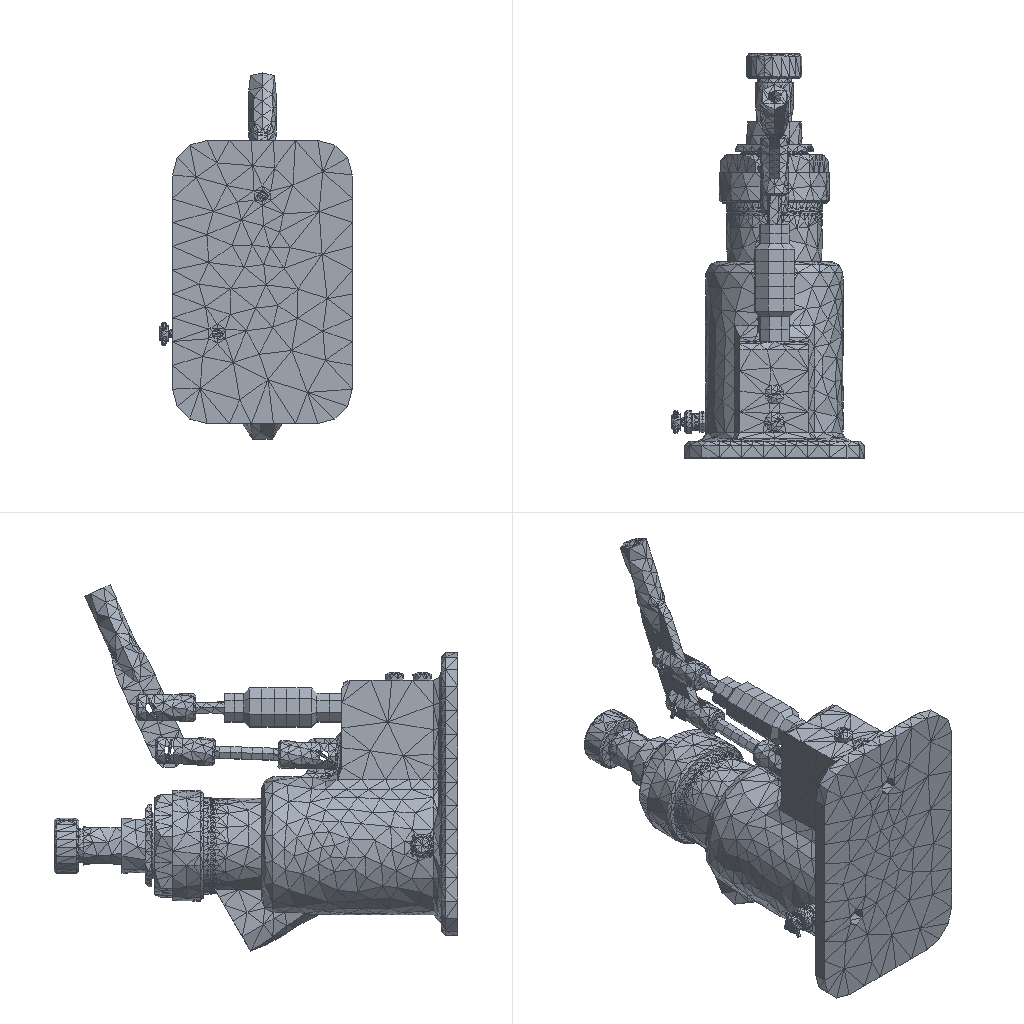Simulation study | ansys workbench
Ansys APDL input file, long lists of numbers shortened:
/batch
/config,noeldb,1     ! force off writing results to database
*get,_wallstrt,active,,time,wall
! ANSYS input file written by Workbench version 2022 R1
! File used for geometry attach:
/title,___--__ (B5)
! ****** Begin Custom Load Command Snippet ******
/COM, ACT Extensions:
/COM,     LSDYNA, 2021.1
/COM,
! ****** End   Custom Load Command Snippet ******
*DIM,_wb_ProjectScratch_dir,string,248
_wb_ProjectScratch_dir(1) = ''
*DIM,_wb_SolverFiles_dir,string,248
_wb_SolverFiles_dir(1) = ''
*DIM,_wb_userfiles_dir,string,248
_wb_userfiles_dir(1) = ''
/com,--- Data in consistent NMM units. See Solving Units in the help system for more information.
/units,MPA
/nopr
/wb,file,start              !  signify a WB generated input file
/prep7
! Turn off shape checking because checks already performed inside WB mesher.
! See help system for more information.
SHPP,OFF,,NOWARN
/nolist
etcon,set             ! allow ANSYS to choose best KEYOP's for 180x elements, resets any applicable keyopt to MAPDL defaults
/com,*********** Nodes for the whole assembly ***********
nblock,3,,64544
(1i9,3e20.9e3)
        1     2.522581875E+01    -4.240918474E+01     1.018764446E+02
! (58676 more lines like these left out)
-1
/wb,elem,start            !  set before creation of elements
/com,*********** Elements for Body 1 "3 - Caixa|Chamfer3" ***********
et,1,187
eblock,19,solid,,12883
(19i9)
        1        1        1        1        0        0        0        0       10        0    15841    34635    35994    34636    35272    49223    49227    49216    49218
! (25765 more lines like these left out)
-1
/com,*********** Elements for Body 2 "4 - Camisa|3/16 (0.1875) Diameter Hole1" ***********
et,2,187
eblock,19,solid,,1067
(19i9)
        2        2        2        2        0        0        0        0       10        0    10106    21478    21481    21733    21857    21878    21894    21881    21882
! (2133 more lines like these left out)
-1
/com,*********** Elements for Body 3 "2 - Porca especial|Cut-Revolve2" ***********
et,3,187
eblock,19,solid,,1009
(19i9)
        3        3        3        3        0        0        0        0       10        0     6814    15045    15047    15293    15279    16019    16039    16027    16025
! (2017 more lines like these left out)
-1
/com,*********** Elements for Body 4 "11 - Porca especial|Chamfer2" ***********
et,4,187
eblock,19,solid,,3371
(19i9)
        4        4        4        4        0        0        0        0       10        0    11173    24012    24701    24402    24248    26827    28868    26825    26824
! (6741 more lines like these left out)
-1
/com,*********** Elements for Body 5 "38 - Eixo Central|Chamfer1" ***********
et,5,187
eblock,19,solid,,853
(19i9)
        5        5        5        5        0        0        0        0       10        0     5961    13343    13573    13546    13550    13911    14889    13907    13908
! (1705 more lines like these left out)
-1
! (22 more sections like these left out)
/wb,elem,end               !  done creating elements
/com,*********** Send User Defined Coordinate System(s) ***********
csys,0
toffst,273.15,  ! Temperature offset from absolute zero
/com,*********** Set Reference Temperature ***********
tref,22.
/wb,mat,start              !  starting to send materials
/com,*********** Send Materials ***********
Temperature = 'TEMP' ! Temperature
MP,DENS,1,7.85e-09,	! tonne mm^-3
MP,ALPX,1,1.2e-05,	! C^-1
MP,C,1,434000000,	! mm^2 s^-2 C^-1
MP,KXX,1,60.5,	! tonne mm s^-3 C^-1
MP,RSVX,1,0.00017,	! ohm mm
MP,EX,1,200000,	! tonne s^-2 mm^-1
MP,NUXY,1,0.3,
MP,MURX,1,10000,
Temperature = 'TEMP' ! Temperature
MP,DENS,2,7.85e-09,	! tonne mm^-3
MP,ALPX,2,1.2e-05,	! C^-1
MP,C,2,434000000,	! mm^2 s^-2 C^-1
MP,KXX,2,60.5,	! tonne mm s^-3 C^-1
MP,RSVX,2,0.00017,	! ohm mm
MP,EX,2,200000,	! tonne s^-2 mm^-1
MP,NUXY,2,0.3,
MP,MURX,2,10000,
Temperature = 'TEMP' ! Temperature
MP,DENS,3,7.85e-09,	! tonne mm^-3
MP,ALPX,3,1.2e-05,	! C^-1
MP,C,3,434000000,	! mm^2 s^-2 C^-1
MP,KXX,3,60.5,	! tonne mm s^-3 C^-1
MP,RSVX,3,0.00017,	! ohm mm
MP,EX,3,200000,	! tonne s^-2 mm^-1
MP,NUXY,3,0.3,
MP,MURX,3,10000,
Temperature = 'TEMP' ! Temperature
MP,DENS,4,7.85e-09,	! tonne mm^-3
MP,ALPX,4,1.2e-05,	! C^-1
MP,C,4,434000000,	! mm^2 s^-2 C^-1
MP,KXX,4,60.5,	! tonne mm s^-3 C^-1
MP,RSVX,4,0.00017,	! ohm mm
MP,EX,4,200000,	! tonne s^-2 mm^-1
MP,NUXY,4,0.3,
MP,MURX,4,10000,
Temperature = 'TEMP' ! Temperature
MP,DENS,5,7.85e-09,	! tonne mm^-3
MP,ALPX,5,1.2e-05,	! C^-1
MP,C,5,434000000,	! mm^2 s^-2 C^-1
MP,KXX,5,60.5,	! tonne mm s^-3 C^-1
MP,RSVX,5,0.00017,	! ohm mm
MP,EX,5,200000,	! tonne s^-2 mm^-1
MP,NUXY,5,0.3,
MP,MURX,5,10000,
Temperature = 'TEMP' ! Temperature
MP,DENS,6,7.85e-09,	! tonne mm^-3
MP,ALPX,6,1.2e-05,	! C^-1
MP,C,6,434000000,	! mm^2 s^-2 C^-1
MP,KXX,6,60.5,	! tonne mm s^-3 C^-1
MP,RSVX,6,0.00017,	! ohm mm
MP,EX,6,200000,	! tonne s^-2 mm^-1
MP,NUXY,6,0.3,
MP,MURX,6,10000,
Temperature = 'TEMP' ! Temperature
MP,DENS,7,7.85e-09,	! tonne mm^-3
MP,ALPX,7,1.2e-05,	! C^-1
MP,C,7,434000000,	! mm^2 s^-2 C^-1
MP,KXX,7,60.5,	! tonne mm s^-3 C^-1
MP,RSVX,7,0.00017,	! ohm mm
MP,EX,7,200000,	! tonne s^-2 mm^-1
MP,NUXY,7,0.3,
MP,MURX,7,10000,
Temperature = 'TEMP' ! Temperature
MP,DENS,8,7.85e-09,	! tonne mm^-3
MP,ALPX,8,1.2e-05,	! C^-1
MP,C,8,434000000,	! mm^2 s^-2 C^-1
MP,KXX,8,60.5,	! tonne mm s^-3 C^-1
MP,RSVX,8,0.00017,	! ohm mm
MP,EX,8,200000,	! tonne s^-2 mm^-1
MP,NUXY,8,0.3,
MP,MURX,8,10000,
Temperature = 'TEMP' ! Temperature
MP,DENS,9,7.85e-09,	! tonne mm^-3
MP,ALPX,9,1.2e-05,	! C^-1
MP,C,9,434000000,	! mm^2 s^-2 C^-1
MP,KXX,9,60.5,	! tonne mm s^-3 C^-1
MP,RSVX,9,0.00017,	! ohm mm
MP,EX,9,200000,	! tonne s^-2 mm^-1
! (164 more lines like these left out)
/wb,mat,end                !  done sending materials
!************************* Model Summary ********************
!3 - Caixa|Chamfer3,	结构钢,	matid,	1
!4 - Camisa|3/16 (0.1875) Diameter Hole1,	结构钢,	matid,	2
!2 - Porca especial|Cut-Revolve2,	结构钢,	matid,	3
!11 - Porca especial|Chamfer2,	结构钢,	matid,	4
!38 - Eixo Central|Chamfer1,	结构钢,	matid,	5
!10 - Espiga|Cut-Extrude1,	结构钢,	matid,	6
!8 - Agulha|Chamfer2,	结构钢,	matid,	7
!9 - Parafuso da agulha|M6 Tapped Hole1,	结构钢,	matid,	8
!7 - Porca Trava|M12 Tapped Hole1,	结构钢,	matid,	9
!23 - Esfera|Revolve1,	结构钢,	matid,	10
!23 - Esfera|Revolve1[2],	结构钢,	matid,	11
!24 - Mola|Cut-Extrude1,	结构钢,	matid,	12
!24 - Mola|Cut-Extrude1[2],	结构钢,	matid,	13
!37 - Encaixa de alavanca|Cut-Extrude3,	结构钢,	matid,	14
!33 - Eixo de encaixe|Boss-Extrude2,	结构钢,	matid,	15
!37 - Encaixa de alavanca|Cut-Extrude3[2],	结构钢,	matid,	16
!36 - Alavanca|_10.0 (10) Diameter Hole1,	结构钢,	matid,	17
!37 - Encaixa de alavanca|Cut-Extrude3[3],	结构钢,	matid,	18
!30 - Eixo Injector|M6 Tapped Hole1,	结构钢,	matid,	19
!socket head cap screw_din_DIN 912 M6 x 20 --- 20N|Hex,	结构钢,	matid,	20
!split pin_din_DIN 94-2x10-C-St|ConeCut,	结构钢,	matid,	21
!split pin_din_DIN 94-2x10-C-St|ConeCut[2],	结构钢,	matid,	22
!split pin_din_DIN 94-2x10-C-St|ConeCut[3],	结构钢,	matid,	23
!22 - Luva do pist_o|_10.0 (10) Diameter Hole1,	结构钢,	matid,	24
!26 - Parafuso cabe_a redonda|Cut-Extrude1,	结构钢,	matid,	25
!26 - Parafuso cabe_a redonda|Cut-Extrude1[2],	结构钢,	matid,	26
!17 - Apoio do _mbolo|Chamfer1,	结构钢,	matid,	27
!************************* End Model Summary ********************
! get the diagonal of the bounding box. Needed later for other things
*get,_xmin,node,,mnloc,x
*get,_ymin,node,,mnloc,y
*get,_zmin,node,,mnloc,z
*get,_xmax,node,,mxloc,x
*get,_ymax,node,,mxloc,y
*get,_zmax,node,,mxloc,z
_ASMDIAG=(_xmax-_xmin)*(_xmax-_xmin)+(_ymax-_ymin)*(_ymax-_ymin)+(_zmax-_zmin)*(_zmax-_zmin)
_ASMDIAG=SQRT(_ASMDIAG)
/wb,contact,start          !  starting to send contact
/com,*********** Create Contact "接触区域" ***********
/com,            Real Constant Set For Above Contact Is 29 & 28
*set,tid,29
*set,cid,28
r,tid
r,cid
et,tid,170
et,cid,174
eblock,10,,,158
(15i9)
    46300       29       29       29        0    32764    32770    32772    32772    38335    38424    32772    38336
! (157 more lines like these left out)
-1
eblock,10,,,158
(15i9)
    46458       28       28       28        0    32764    32770    32772    32772    38335    38424    32772    38336
! (157 more lines like these left out)
-1
eblock,10,,,97
(15i9)
    46616       28       29       28        0    21490    21491    21604    21604    21941    21947    21604    21944
! (96 more lines like these left out)
-1
eblock,10,,,97
(15i9)
    46713       29       28       29        0    21490    21491    21604    21604    21941    21947    21604    21944
! (96 more lines like these left out)
-1
keyo,cid,8,2               ! auto create asymmetric contact (from Program Controlled setting)
keyo,cid,10,0              ! adjust contact stiffness each NR iteration (from Program Controlled setting)
keyo,cid,12,5              ! bonded always
keyo,cid,18,1              ! small sliding turned on by application
keyo,cid,2,0               ! augmented Lagrange (from Program Controlled setting)
keyo,cid,4,0               ! on Gauss point (from Program Controlled setting)
keyo,cid,9,1               ! ignore initial gaps/penetration
keyo,cid,7,0               ! No Prediction
rmod,tid,3,10.      ! FKN
rmod,tid,5,0.       ! ICONT
rmod,tid,6,0.       ! PINB
rmod,tid,10,0.      ! CNOF
rmod,tid,12,0.      ! FKT
rmod,tid,36,104     ! WB DSID
rmod,cid,3,10.      ! FKN
rmod,cid,5,0.       ! ICONT
rmod,cid,6,0.       ! PINB
rmod,cid,10,0.      ! CNOF
rmod,cid,12,0.      ! FKT
rmod,cid,36,104     ! WB DSID
/com,*********** Create Contact "接触区域 2" ***********
/com,            Real Constant Set For Above Contact Is 31 & 30
*set,tid,31
*set,cid,30
r,tid
r,cid
et,tid,170
et,cid,174
eblock,10,,,61
(15i9)
    46810       31       31       31        0    32608    32607    34212    34212    37151    37154    34212    37162
! (60 more lines like these left out)
-1
eblock,10,,,61
(15i9)
    46871       30       30       30        0    32608    32607    34212    34212    37151    37154    34212    37162
! (60 more lines like these left out)
-1
eblock,10,,,24
(15i9)
    46932       30       31       30        0     7095     7094     7098     7098     8107     8108     7098     8112
! (23 more lines like these left out)
-1
eblock,10,,,24
(15i9)
    46956       31       30       31        0     7095     7094     7098     7098     8107     8108     7098     8112
! (23 more lines like these left out)
-1
keyo,cid,8,2               ! auto create asymmetric contact (from Program Controlled setting)
keyo,cid,10,0              ! adjust contact stiffness each NR iteration (from Program Controlled setting)
keyo,cid,12,5              ! bonded always
keyo,cid,18,1              ! small sliding turned on by application
keyo,cid,2,0               ! augmented Lagrange (from Program Controlled setting)
keyo,cid,4,0               ! on Gauss point (from Program Controlled setting)
keyo,cid,9,1               ! ignore initial gaps/penetration
keyo,cid,7,0               ! No Prediction
rmod,tid,3,10.      ! FKN
rmod,tid,5,0.       ! ICONT
rmod,tid,6,0.       ! PINB
rmod,tid,10,0.      ! CNOF
rmod,tid,12,0.      ! FKT
rmod,tid,36,107     ! WB DSID
rmod,cid,3,10.      ! FKN
rmod,cid,5,0.       ! ICONT
rmod,cid,6,0.       ! PINB
rmod,cid,10,0.      ! CNOF
rmod,cid,12,0.      ! FKT
rmod,cid,36,107     ! WB DSID
/com,*********** Create Contact "接触区域 3" ***********
/com,            Real Constant Set For Above Contact Is 33 & 32
*set,tid,33
*set,cid,32
r,tid
r,cid
et,tid,170
et,cid,174
eblock,10,,,18
(15i9)
    46980       33       33       33        0    32663    32664    33259    33259    37561    37568    33259    37562
! (17 more lines like these left out)
-1
eblock,10,,,18
(15i9)
    46998       32       32       32        0    32663    32664    33259    33259    37561    37568    33259    37562
! (17 more lines like these left out)
-1
eblock,10,,,16
(15i9)
    47016       32       33       32        0     4137     4136     4124     4124     4251     4218     4124     4219
! (15 more lines like these left out)
-1
eblock,10,,,16
(15i9)
    47032       33       32       33        0     4137     4136     4124     4124     4251     4218     4124     4219
! (15 more lines like these left out)
-1
keyo,cid,8,2               ! auto create asymmetric contact (from Program Controlled setting)
keyo,cid,10,0              ! adjust contact stiffness each NR iteration (from Program Controlled setting)
keyo,cid,12,5              ! bonded always
keyo,cid,18,1              ! small sliding turned on by application
keyo,cid,2,0               ! augmented Lagrange (from Program Controlled setting)
keyo,cid,4,0               ! on Gauss point (from Program Controlled setting)
keyo,cid,9,1               ! ignore initial gaps/penetration
keyo,cid,7,0               ! No Prediction
rmod,tid,3,10.      ! FKN
rmod,tid,5,0.       ! ICONT
rmod,tid,6,0.       ! PINB
rmod,tid,10,0.      ! CNOF
rmod,tid,12,0.      ! FKT
rmod,tid,36,110     ! WB DSID
rmod,cid,3,10.      ! FKN
rmod,cid,5,0.       ! ICONT
rmod,cid,6,0.       ! PINB
rmod,cid,10,0.      ! CNOF
rmod,cid,12,0.      ! FKT
rmod,cid,36,110     ! WB DSID
/com,*********** Create Contact "接触区域 4" ***********
/com,            Real Constant Set For Above Contact Is 35 & 34
*set,tid,35
*set,cid,34
r,tid
r,cid
et,tid,170
et,cid,174
eblock,10,,,49
(15i9)
    47048       35       35       35        0    32673    34235    32683    32683    37624    37703    32683    37622
! (48 more lines like these left out)
-1
eblock,10,,,49
(15i9)
    47097       34       34       34        0    32673    34235    32683    32683    37624    37703    32683    37622
! (48 more lines like these left out)
-1
eblock,10,,,122
(15i9)
    47146       34       35       34        0     3721     3722     3752     3752     3855     3864     3752     3858
! (121 more lines like these left out)
-1
eblock,10,,,122
(15i9)
    47268       35       34       35        0     3721     3722     3752     3752     3855     3864     3752     3858
! (121 more lines like these left out)
-1
keyo,cid,8,2               ! auto create asymmetric contact (from Program Controlled setting)
keyo,cid,10,0              ! adjust contact stiffness each NR iteration (from Program Controlled setting)
keyo,cid,12,5              ! bonded always
keyo,cid,18,1              ! small sliding turned on by application
keyo,cid,2,0               ! augmented Lagrange (from Program Controlled setting)
keyo,cid,4,0               ! on Gauss point (from Program Controlled setting)
keyo,cid,9,1               ! ignore initial gaps/penetration
keyo,cid,7,0               ! No Prediction
rmod,tid,3,10.      ! FKN
rmod,tid,5,0.       ! ICONT
rmod,tid,6,0.       ! PINB
rmod,tid,10,0.      ! CNOF
rmod,tid,12,0.      ! FKT
rmod,tid,36,113     ! WB DSID
rmod,cid,3,10.      ! FKN
rmod,cid,5,0.       ! ICONT
rmod,cid,6,0.       ! PINB
rmod,cid,10,0.      ! CNOF
rmod,cid,12,0.      ! FKT
rmod,cid,36,113     ! WB DSID
/com,*********** Create Contact "接触区域 5" ***********
/com,            Real Constant Set For Above Contact Is 37 & 36
*set,tid,37
*set,cid,36
r,tid
r,cid
et,tid,170
et,cid,174
eblock,10,,,36
(15i9)
    47390       37       37       37        0    32722    32723    34251    34251    38009    38020    34251    38013
! (35 more lines like these left out)
-1
eblock,10,,,36
(15i9)
    47426       36       36       36        0    32722    32723    34251    34251    38009    38020    34251    38013
! (35 more lines like these left out)
-1
eblock,10,,,122
(15i9)
    47462       36       37       36        0       13       14       44       44      147      156       44      150
! (121 more lines like these left out)
-1
eblock,10,,,122
(15i9)
    47584       37       36       37        0       13       14       44       44      147      156       44      150
! (121 more lines like these left out)
-1
keyo,cid,8,2               ! auto create asymmetric contact (from Program Controlled setting)
keyo,cid,10,0              ! adjust contact stiffness each NR iteration (from Program Controlled setting)
keyo,cid,12,5              ! bonded always
keyo,cid,18,1              ! small sliding turned on by application
keyo,cid,2,0               ! augmented Lagrange (from Program Controlled setting)
keyo,cid,4,0               ! on Gauss point (from Program Controlled setting)
keyo,cid,9,1               ! ignore initial gaps/penetration
keyo,cid,7,0               ! No Prediction
rmod,tid,3,10.      ! FKN
rmod,tid,5,0.       ! ICONT
rmod,tid,6,0.       ! PINB
rmod,tid,10,0.      ! CNOF
rmod,tid,12,0.      ! FKT
rmod,tid,36,116     ! WB DSID
rmod,cid,3,10.      ! FKN
rmod,cid,5,0.       ! ICONT
rmod,cid,6,0.       ! PINB
rmod,cid,10,0.      ! CNOF
rmod,cid,12,0.      ! FKT
rmod,cid,36,116     ! WB DSID
! (24 more sections like these left out)
/wb,contact,end            !  done creating contacts
/golist
/wb,load,start             !  starting to send loads
/gst,on,on
fini
*get,_numnode,node,0,count
*get,_numelem,elem,0,count
*get, _MAXELEMNUM, elem, 0, NUM, MAX
*get, _MAXNODENUM, node, 0, NUM, MAX
*get, _MAXELEMTYPE, etyp, 0, NUM, MAX
*get, _MAXREALCONST, real, 0, NUM, MAX
/go
/wb,load,end               !  done creating loads
/com,--- Number of total nodes = %_numnode%
/com,--- Number of contact elements = 9606
/com,--- Number of spring elements = 0
/com,--- Number of bearing elements = 0
/com,--- Number of solid elements = 30077
/com,--- Number of condensed parts = 0
/com,--- Number of total elements = %_numelem%
*get,_wallbsol,active,,time,wall
/solu
antype,2                   ! modal analysis
_thickRatio=0.444   ! Ratio of thick parts in the model
modopt,lanb,30
outres,erase
outres,all,none
outres,nsol,all
outres,etmp,all
mxpand                    ! default expand in case of complex solution
dmpopt,esav,no
dmpopt,emat,no
dmpopt,full,no
! *********** WB SOLVE COMMAND ***********
! check interactive state
*get,ANSINTER_,active,,int
*if,ANSINTER_,ne,0,then
/eof
*endif
solve
/com *************** Write FE CONNECTORS *********
CEWRITE,file,ce,,INTE
*get,_nmodalsolproc,active,0,numcpu
fini
/nopr
*get,_numnode,node,0,count
*get,_numelem,elem,0,count
*get, _MAXELEMNUM, elem, 0, NUM, MAX
*get, _MAXNODENUM, node, 0, NUM, MAX,,,INTERNAL
*get, _MAXELEMTYPE, etyp, 0, NUM, MAX
*get, _MAXREALCONST, real, 0, NUM, MAX
/gopr
*get,_wallasol,active,,time,wall
/post1
/nopr
*dim,_direction,CHAR,6,1
_direction(1) = 'X'
_direction(2) = 'Y'
_direction(3) = 'Z'
_direction(4) = 'ROTX'
_direction(5) = 'ROTY'
_direction(6) = 'ROTZ'
*get,_lastLS,active,0,set,LSTP
*get,_beginset,active,0,set,nset,first,_lastLS
*get,_endset,active,0,set,nset,last,_lastLS
_nummodes = 0
*if,_endset,gt,0,then
_nummodes = _endset - _beginset + 1
*endif
*do,i_mode,1,_nummodes
   *do,j_component,1,6
			*get,PFACT_%i_mode%_%j_component%,MODE,%i_mode%,PFACT,,DIREC,_direction(%j_component%)
   *enddo
*enddo
*dim,_tmdirection,CHAR,6,1
_tmdirection(1) = 'X'
_tmdirection(2) = 'Y'
_tmdirection(3) = 'Z'
_tmdirection(4) = 'X'
_tmdirection(5) = 'Y'
_tmdirection(6) = 'Z'
*do,j_component,1,6
    *if,j_component,gt,3,then
        *get,TOTALMASS_%j_component%,ELEM,0,IOR,_tmdirection(%j_component%)
    *else
        *get,TOTALMASS_%j_component%,ELEM,0,MTOT,_tmdirection(%j_component%)
    *endif
*enddo
/gopr
xmlo,ENCODING,ISO-8859-1
xmlo,parm
/xml,parm,xml
fini
/gopr
*get,_walldone,active,,time,wall
_preptime=(_wallbsol-_wallstrt)*3600
_solvtime=(_wallasol-_wallbsol)*3600
_posttime=(_walldone-_wallasol)*3600
_totaltim=(_walldone-_wallstrt)*3600
*get,_dlbratio,active,0,solu,dlbr
*get,_combtime,active,0,solu,comb
*get,_ssmode,active,0,solu,ssmm
*get,_ndofs,active,0,solu,ndof
/fclean				!clean distributed files
/com,--- Total number of nodes = %_numnode%
/com,--- Total number of elements = %_numelem%
/com,--- Element load balance ratio = %_dlbratio%
/com,--- Time to combine distributed files = %_combtime%
/com,--- Sparse memory mode = %_ssmode%
/com,--- Number of DOF = %_ndofs%
/wb,file,end               ! done with WB generated input